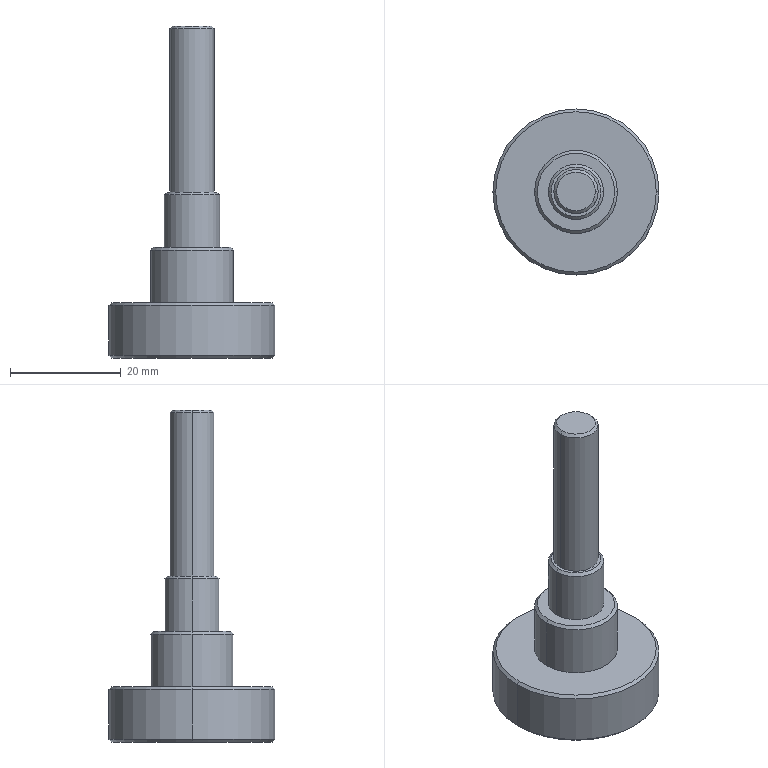Part | SolidWorks | features ICE 3, Chamfer 1, Extrusion 1 | 1 solid | 23 faces | box 30 x 30 x 60 mm | volume 11093 mm3 | cone 10 | cylinder 8 | plane 5 | commonest cylinder face diameters 8 x2 10 x2 15 x2 30 x2
STEP:
#1=CARTESIAN_POINT('',(3.5,0.,60.));
#2=VERTEX_POINT('',#1);
#3=CARTESIAN_POINT('',(-3.5,0.,60.));
#4=VERTEX_POINT('',#3);
#5=CARTESIAN_POINT('',(0.,0.,60.));
#6=DIRECTION('',(0.,0.,1.));
#7=DIRECTION('',(1.,0.,0.));
#8=AXIS2_PLACEMENT_3D('',#5,#6,#7);
#9=CIRCLE('',#8,3.5);
#10=EDGE_CURVE('',#2,#4,#9,.T.);
#11=ORIENTED_EDGE('',*,*,#10,.F.);
#12=CARTESIAN_POINT('',(4.,0.,59.5));
#13=VERTEX_POINT('',#12);
#14=CARTESIAN_POINT('',(3.5,0.,60.));
#15=DIRECTION('',(0.7071,0.,-0.7071));
#16=VECTOR('',#15,1000.);
#17=LINE('',#14,#16);
#18=EDGE_CURVE('',#2,#13,#17,.T.);
#19=ORIENTED_EDGE('',*,*,#18,.T.);
#20=CARTESIAN_POINT('',(-4.,0.,59.5));
#21=VERTEX_POINT('',#20);
#22=CARTESIAN_POINT('',(0.,0.,59.5));
#23=DIRECTION('',(0.,0.,-1.));
#24=DIRECTION('',(1.,0.,0.));
#25=AXIS2_PLACEMENT_3D('',#22,#23,#24);
#26=CIRCLE('',#25,4.);
#27=EDGE_CURVE('',#21,#13,#26,.T.);
#28=ORIENTED_EDGE('',*,*,#27,.F.);
#29=CARTESIAN_POINT('',(-3.5,0.,60.));
#30=DIRECTION('',(-0.7071,0.,-0.7071));
#31=VECTOR('',#30,1000.);
#32=LINE('',#29,#31);
#33=EDGE_CURVE('',#4,#21,#32,.T.);
#34=ORIENTED_EDGE('',*,*,#33,.F.);
#35=EDGE_LOOP('',(#11,#19,#28,#34));
#36=FACE_OUTER_BOUND('',#35,.T.);
#37=CARTESIAN_POINT('',(0.,0.,60.));
#38=DIRECTION('',(0.,0.,-1.));
#39=DIRECTION('',(-1.,0.,0.));
#40=AXIS2_PLACEMENT_3D('',#37,#38,#39);
#41=CONICAL_SURFACE('',#40,3.5,0.7854);
#42=ADVANCED_FACE('',(#36),#41,.T.);
#43=CARTESIAN_POINT('',(4.5,0.,30.));
#44=VERTEX_POINT('',#43);
#45=CARTESIAN_POINT('',(-4.5,0.,30.));
#46=VERTEX_POINT('',#45);
#47=CARTESIAN_POINT('',(0.,0.,30.));
#48=DIRECTION('',(0.,0.,1.));
#49=DIRECTION('',(1.,0.,0.));
#50=AXIS2_PLACEMENT_3D('',#47,#48,#49);
#51=CIRCLE('',#50,4.5);
#52=EDGE_CURVE('',#44,#46,#51,.T.);
#53=ORIENTED_EDGE('',*,*,#52,.F.);
#54=CARTESIAN_POINT('',(5.,0.,29.5));
#55=VERTEX_POINT('',#54);
#56=CARTESIAN_POINT('',(4.5,0.,30.));
#57=DIRECTION('',(0.7071,0.,-0.7071));
#58=VECTOR('',#57,1000.);
#59=LINE('',#56,#58);
#60=EDGE_CURVE('',#44,#55,#59,.T.);
#61=ORIENTED_EDGE('',*,*,#60,.T.);
#62=CARTESIAN_POINT('',(-5.,0.,29.5));
#63=VERTEX_POINT('',#62);
#64=CARTESIAN_POINT('',(0.,0.,29.5));
#65=DIRECTION('',(0.,0.,-1.));
#66=DIRECTION('',(1.,0.,0.));
#67=AXIS2_PLACEMENT_3D('',#64,#65,#66);
#68=CIRCLE('',#67,5.);
#69=EDGE_CURVE('',#63,#55,#68,.T.);
#70=ORIENTED_EDGE('',*,*,#69,.F.);
#71=CARTESIAN_POINT('',(-4.5,0.,30.));
#72=DIRECTION('',(-0.7071,0.,-0.7071));
#73=VECTOR('',#72,1000.);
#74=LINE('',#71,#73);
#75=EDGE_CURVE('',#46,#63,#74,.T.);
#76=ORIENTED_EDGE('',*,*,#75,.F.);
#77=EDGE_LOOP('',(#53,#61,#70,#76));
#78=FACE_OUTER_BOUND('',#77,.T.);
#79=CARTESIAN_POINT('',(0.,0.,30.));
#80=DIRECTION('',(0.,0.,-1.));
#81=DIRECTION('',(-1.,0.,0.));
#82=AXIS2_PLACEMENT_3D('',#79,#80,#81);
#83=CONICAL_SURFACE('',#82,4.5,0.7854);
#84=ADVANCED_FACE('',(#78),#83,.T.);
#85=CARTESIAN_POINT('',(7.,0.,20.));
#86=VERTEX_POINT('',#85);
#87=CARTESIAN_POINT('',(-7.,0.,20.));
#88=VERTEX_POINT('',#87);
#89=CARTESIAN_POINT('',(0.,0.,20.));
#90=DIRECTION('',(0.,0.,1.));
#91=DIRECTION('',(1.,0.,0.));
#92=AXIS2_PLACEMENT_3D('',#89,#90,#91);
#93=CIRCLE('',#92,7.);
#94=EDGE_CURVE('',#86,#88,#93,.T.);
#95=ORIENTED_EDGE('',*,*,#94,.F.);
#96=CARTESIAN_POINT('',(7.5,0.,19.5));
#97=VERTEX_POINT('',#96);
#98=CARTESIAN_POINT('',(7.,0.,20.));
#99=DIRECTION('',(0.7071,0.,-0.7071));
#100=VECTOR('',#99,1000.);
#101=LINE('',#98,#100);
#102=EDGE_CURVE('',#86,#97,#101,.T.);
#103=ORIENTED_EDGE('',*,*,#102,.T.);
#104=CARTESIAN_POINT('',(-7.5,0.,19.5));
#105=VERTEX_POINT('',#104);
#106=CARTESIAN_POINT('',(0.,0.,19.5));
#107=DIRECTION('',(0.,0.,-1.));
#108=DIRECTION('',(1.,0.,0.));
#109=AXIS2_PLACEMENT_3D('',#106,#107,#108);
#110=CIRCLE('',#109,7.5);
#111=EDGE_CURVE('',#105,#97,#110,.T.);
#112=ORIENTED_EDGE('',*,*,#111,.F.);
#113=CARTESIAN_POINT('',(-7.,0.,20.));
#114=DIRECTION('',(-0.7071,0.,-0.7071));
#115=VECTOR('',#114,1000.);
#116=LINE('',#113,#115);
#117=EDGE_CURVE('',#88,#105,#116,.T.);
#118=ORIENTED_EDGE('',*,*,#117,.F.);
#119=EDGE_LOOP('',(#95,#103,#112,#118));
#120=FACE_OUTER_BOUND('',#119,.T.);
#121=CARTESIAN_POINT('',(0.,0.,20.));
#122=DIRECTION('',(0.,0.,-1.));
#123=DIRECTION('',(-1.,0.,0.));
#124=AXIS2_PLACEMENT_3D('',#121,#122,#123);
#125=CONICAL_SURFACE('',#124,7.,0.7854);
#126=ADVANCED_FACE('',(#120),#125,.T.);
#127=CARTESIAN_POINT('',(14.5,0.,10.));
#128=VERTEX_POINT('',#127);
#129=CARTESIAN_POINT('',(-14.5,0.,10.));
#130=VERTEX_POINT('',#129);
#131=CARTESIAN_POINT('',(0.,0.,10.));
#132=DIRECTION('',(0.,0.,1.));
#133=DIRECTION('',(1.,0.,0.));
#134=AXIS2_PLACEMENT_3D('',#131,#132,#133);
#135=CIRCLE('',#134,14.5);
#136=EDGE_CURVE('',#128,#130,#135,.T.);
#137=ORIENTED_EDGE('',*,*,#136,.F.);
#138=CARTESIAN_POINT('',(15.,0.,9.5));
#139=VERTEX_POINT('',#138);
#140=CARTESIAN_POINT('',(14.5,0.,10.));
#141=DIRECTION('',(0.7071,0.,-0.7071));
#142=VECTOR('',#141,1000.);
#143=LINE('',#140,#142);
#144=EDGE_CURVE('',#128,#139,#143,.T.);
#145=ORIENTED_EDGE('',*,*,#144,.T.);
#146=CARTESIAN_POINT('',(-15.,0.,9.5));
#147=VERTEX_POINT('',#146);
#148=CARTESIAN_POINT('',(0.,0.,9.5));
#149=DIRECTION('',(0.,0.,-1.));
#150=DIRECTION('',(1.,0.,0.));
#151=AXIS2_PLACEMENT_3D('',#148,#149,#150);
#152=CIRCLE('',#151,15.);
#153=EDGE_CURVE('',#147,#139,#152,.T.);
#154=ORIENTED_EDGE('',*,*,#153,.F.);
#155=CARTESIAN_POINT('',(-14.5,0.,10.));
#156=DIRECTION('',(-0.7071,0.,-0.7071));
#157=VECTOR('',#156,1000.);
#158=LINE('',#155,#157);
#159=EDGE_CURVE('',#130,#147,#158,.T.);
#160=ORIENTED_EDGE('',*,*,#159,.F.);
#161=EDGE_LOOP('',(#137,#145,#154,#160));
#162=FACE_OUTER_BOUND('',#161,.T.);
#163=CARTESIAN_POINT('',(0.,0.,10.));
#164=DIRECTION('',(0.,0.,-1.));
#165=DIRECTION('',(-1.,0.,0.));
#166=AXIS2_PLACEMENT_3D('',#163,#164,#165);
#167=CONICAL_SURFACE('',#166,14.5,0.7854);
#168=ADVANCED_FACE('',(#162),#167,.T.);
#169=CARTESIAN_POINT('',(-14.5,0.,0.));
#170=VERTEX_POINT('',#169);
#171=CARTESIAN_POINT('',(14.5,0.,0.));
#172=VERTEX_POINT('',#171);
#173=CARTESIAN_POINT('',(0.,0.,0.));
#174=DIRECTION('',(0.,0.,-1.));
#175=DIRECTION('',(1.,0.,0.));
#176=AXIS2_PLACEMENT_3D('',#173,#174,#175);
#177=CIRCLE('',#176,14.5);
#178=EDGE_CURVE('',#170,#172,#177,.T.);
#179=ORIENTED_EDGE('',*,*,#178,.F.);
#180=CARTESIAN_POINT('',(-15.,0.,0.5));
#181=VERTEX_POINT('',#180);
#182=CARTESIAN_POINT('',(-15.,0.,0.5));
#183=DIRECTION('',(-0.7071,0.,0.7071));
#184=VECTOR('',#183,1000.);
#185=LINE('',#182,#184);
#186=EDGE_CURVE('',#170,#181,#185,.T.);
#187=ORIENTED_EDGE('',*,*,#186,.T.);
#188=CARTESIAN_POINT('',(15.,0.,0.5));
#189=VERTEX_POINT('',#188);
#190=CARTESIAN_POINT('',(0.,0.,0.5));
#191=DIRECTION('',(0.,0.,1.));
#192=DIRECTION('',(1.,0.,0.));
#193=AXIS2_PLACEMENT_3D('',#190,#191,#192);
#194=CIRCLE('',#193,15.);
#195=EDGE_CURVE('',#189,#181,#194,.T.);
#196=ORIENTED_EDGE('',*,*,#195,.F.);
#197=CARTESIAN_POINT('',(15.,0.,0.5));
#198=DIRECTION('',(0.7071,0.,0.7071));
#199=VECTOR('',#198,1000.);
#200=LINE('',#197,#199);
#201=EDGE_CURVE('',#172,#189,#200,.T.);
#202=ORIENTED_EDGE('',*,*,#201,.F.);
#203=EDGE_LOOP('',(#179,#187,#196,#202));
#204=FACE_OUTER_BOUND('',#203,.T.);
#205=CARTESIAN_POINT('',(0.,0.,0.5));
#206=DIRECTION('',(0.,0.,1.));
#207=DIRECTION('',(1.,0.,0.));
#208=AXIS2_PLACEMENT_3D('',#205,#206,#207);
#209=CONICAL_SURFACE('',#208,15.,0.7854);
#210=ADVANCED_FACE('',(#204),#209,.T.);
#211=ORIENTED_EDGE('',*,*,#27,.T.);
#212=CARTESIAN_POINT('',(4.,0.,30.));
#213=VERTEX_POINT('',#212);
#214=CARTESIAN_POINT('',(4.,0.,60.));
#215=DIRECTION('',(0.,0.,-1.));
#216=VECTOR('',#215,1000.);
#217=LINE('',#214,#216);
#218=EDGE_CURVE('',#13,#213,#217,.T.);
#219=ORIENTED_EDGE('',*,*,#218,.T.);
#220=CARTESIAN_POINT('',(-4.,0.,30.));
#221=VERTEX_POINT('',#220);
#222=CARTESIAN_POINT('',(0.,0.,30.));
#223=DIRECTION('',(0.,0.,1.));
#224=DIRECTION('',(1.,0.,0.));
#225=AXIS2_PLACEMENT_3D('',#222,#223,#224);
#226=CIRCLE('',#225,4.);
#227=EDGE_CURVE('',#213,#221,#226,.T.);
#228=ORIENTED_EDGE('',*,*,#227,.T.);
#229=CARTESIAN_POINT('',(-4.,0.,60.));
#230=DIRECTION('',(0.,0.,-1.));
#231=VECTOR('',#230,1000.);
#232=LINE('',#229,#231);
#233=EDGE_CURVE('',#21,#221,#232,.T.);
#234=ORIENTED_EDGE('',*,*,#233,.F.);
#235=EDGE_LOOP('',(#211,#219,#228,#234));
#236=FACE_OUTER_BOUND('',#235,.T.);
#237=CARTESIAN_POINT('',(0.,0.,60.));
#238=DIRECTION('',(0.,0.,-1.));
#239=DIRECTION('',(-1.,0.,0.));
#240=AXIS2_PLACEMENT_3D('',#237,#238,#239);
#241=CYLINDRICAL_SURFACE('',#240,4.);
#242=ADVANCED_FACE('',(#236),#241,.T.);
#243=ORIENTED_EDGE('',*,*,#69,.T.);
#244=CARTESIAN_POINT('',(5.,0.,20.));
#245=VERTEX_POINT('',#244);
#246=CARTESIAN_POINT('',(5.,0.,30.));
#247=DIRECTION('',(0.,0.,-1.));
#248=VECTOR('',#247,1000.);
#249=LINE('',#246,#248);
#250=EDGE_CURVE('',#55,#245,#249,.T.);
#251=ORIENTED_EDGE('',*,*,#250,.T.);
#252=CARTESIAN_POINT('',(-5.,0.,20.));
#253=VERTEX_POINT('',#252);
#254=CARTESIAN_POINT('',(0.,0.,20.));
#255=DIRECTION('',(0.,0.,1.));
#256=DIRECTION('',(1.,0.,0.));
#257=AXIS2_PLACEMENT_3D('',#254,#255,#256);
#258=CIRCLE('',#257,5.);
#259=EDGE_CURVE('',#245,#253,#258,.T.);
#260=ORIENTED_EDGE('',*,*,#259,.T.);
#261=CARTESIAN_POINT('',(-5.,0.,30.));
#262=DIRECTION('',(0.,0.,-1.));
#263=VECTOR('',#262,1000.);
#264=LINE('',#261,#263);
#265=EDGE_CURVE('',#63,#253,#264,.T.);
#266=ORIENTED_EDGE('',*,*,#265,.F.);
#267=EDGE_LOOP('',(#243,#251,#260,#266));
#268=FACE_OUTER_BOUND('',#267,.T.);
#269=CARTESIAN_POINT('',(0.,0.,30.));
#270=DIRECTION('',(0.,0.,-1.));
#271=DIRECTION('',(-1.,0.,0.));
#272=AXIS2_PLACEMENT_3D('',#269,#270,#271);
#273=CYLINDRICAL_SURFACE('',#272,5.);
#274=ADVANCED_FACE('',(#268),#273,.T.);
#275=ORIENTED_EDGE('',*,*,#111,.T.);
#276=CARTESIAN_POINT('',(7.5,0.,10.));
#277=VERTEX_POINT('',#276);
#278=CARTESIAN_POINT('',(7.5,0.,20.));
#279=DIRECTION('',(0.,0.,-1.));
#280=VECTOR('',#279,1000.);
#281=LINE('',#278,#280);
#282=EDGE_CURVE('',#97,#277,#281,.T.);
#283=ORIENTED_EDGE('',*,*,#282,.T.);
#284=CARTESIAN_POINT('',(-7.5,0.,10.));
#285=VERTEX_POINT('',#284);
#286=CARTESIAN_POINT('',(0.,0.,10.));
#287=DIRECTION('',(0.,0.,1.));
#288=DIRECTION('',(1.,0.,0.));
#289=AXIS2_PLACEMENT_3D('',#286,#287,#288);
#290=CIRCLE('',#289,7.5);
#291=EDGE_CURVE('',#277,#285,#290,.T.);
#292=ORIENTED_EDGE('',*,*,#291,.T.);
#293=CARTESIAN_POINT('',(-7.5,0.,20.));
#294=DIRECTION('',(0.,0.,-1.));
#295=VECTOR('',#294,1000.);
#296=LINE('',#293,#295);
#297=EDGE_CURVE('',#105,#285,#296,.T.);
#298=ORIENTED_EDGE('',*,*,#297,.F.);
#299=EDGE_LOOP('',(#275,#283,#292,#298));
#300=FACE_OUTER_BOUND('',#299,.T.);
#301=CARTESIAN_POINT('',(0.,0.,20.));
#302=DIRECTION('',(0.,0.,-1.));
#303=DIRECTION('',(-1.,0.,0.));
#304=AXIS2_PLACEMENT_3D('',#301,#302,#303);
#305=CYLINDRICAL_SURFACE('',#304,7.5);
#306=ADVANCED_FACE('',(#300),#305,.T.);
#307=ORIENTED_EDGE('',*,*,#153,.T.);
#308=CARTESIAN_POINT('',(15.,0.,10.));
#309=DIRECTION('',(0.,0.,-1.));
#310=VECTOR('',#309,1000.);
#311=LINE('',#308,#310);
#312=EDGE_CURVE('',#139,#189,#311,.T.);
#313=ORIENTED_EDGE('',*,*,#312,.T.);
#314=ORIENTED_EDGE('',*,*,#195,.T.);
#315=CARTESIAN_POINT('',(-15.,0.,10.));
#316=DIRECTION('',(0.,0.,-1.));
#317=VECTOR('',#316,1000.);
#318=LINE('',#315,#317);
#319=EDGE_CURVE('',#147,#181,#318,.T.);
#320=ORIENTED_EDGE('',*,*,#319,.F.);
#321=EDGE_LOOP('',(#307,#313,#314,#320));
#322=FACE_OUTER_BOUND('',#321,.T.);
#323=CARTESIAN_POINT('',(0.,0.,10.));
#324=DIRECTION('',(0.,0.,-1.));
#325=DIRECTION('',(-1.,0.,0.));
#326=AXIS2_PLACEMENT_3D('',#323,#324,#325);
#327=CYLINDRICAL_SURFACE('',#326,15.);
#328=ADVANCED_FACE('',(#322),#327,.T.);
#329=CARTESIAN_POINT('',(0.,0.,20.));
#330=DIRECTION('',(0.,0.,1.));
#331=DIRECTION('',(1.,0.,0.));
#332=AXIS2_PLACEMENT_3D('',#329,#330,#331);
#333=CIRCLE('',#332,7.);
#334=EDGE_CURVE('',#88,#86,#333,.T.);
#335=ORIENTED_EDGE('',*,*,#334,.T.);
#336=ORIENTED_EDGE('',*,*,#94,.T.);
#337=EDGE_LOOP('',(#335,#336));
#338=FACE_OUTER_BOUND('',#337,.T.);
#339=CARTESIAN_POINT('',(0.,0.,20.));
#340=DIRECTION('',(0.,0.,1.));
#341=DIRECTION('',(1.,0.,0.));
#342=AXIS2_PLACEMENT_3D('',#339,#340,#341);
#343=CIRCLE('',#342,5.);
#344=EDGE_CURVE('',#253,#245,#343,.T.);
#345=ORIENTED_EDGE('',*,*,#344,.F.);
#346=ORIENTED_EDGE('',*,*,#259,.F.);
#347=EDGE_LOOP('',(#345,#346));
#348=FACE_BOUND('',#347,.T.);
#349=CARTESIAN_POINT('',(0.,0.,20.));
#350=DIRECTION('',(0.,0.,1.));
#351=DIRECTION('',(1.,0.,0.));
#352=AXIS2_PLACEMENT_3D('',#349,#350,#351);
#353=PLANE('',#352);
#354=ADVANCED_FACE('',(#338,#348),#353,.T.);
#355=CARTESIAN_POINT('',(0.,0.,10.));
#356=DIRECTION('',(0.,0.,1.));
#357=DIRECTION('',(1.,0.,0.));
#358=AXIS2_PLACEMENT_3D('',#355,#356,#357);
#359=CIRCLE('',#358,14.5);
#360=EDGE_CURVE('',#130,#128,#359,.T.);
#361=ORIENTED_EDGE('',*,*,#360,.T.);
#362=ORIENTED_EDGE('',*,*,#136,.T.);
#363=EDGE_LOOP('',(#361,#362));
#364=FACE_OUTER_BOUND('',#363,.T.);
#365=CARTESIAN_POINT('',(0.,0.,10.));
#366=DIRECTION('',(0.,0.,1.));
#367=DIRECTION('',(1.,0.,0.));
#368=AXIS2_PLACEMENT_3D('',#365,#366,#367);
#369=CIRCLE('',#368,7.5);
#370=EDGE_CURVE('',#285,#277,#369,.T.);
#371=ORIENTED_EDGE('',*,*,#370,.F.);
#372=ORIENTED_EDGE('',*,*,#291,.F.);
#373=EDGE_LOOP('',(#371,#372));
#374=FACE_BOUND('',#373,.T.);
#375=CARTESIAN_POINT('',(0.,0.,10.));
#376=DIRECTION('',(0.,0.,1.));
#377=DIRECTION('',(1.,0.,0.));
#378=AXIS2_PLACEMENT_3D('',#375,#376,#377);
#379=PLANE('',#378);
#380=ADVANCED_FACE('',(#364,#374),#379,.T.);
#381=ORIENTED_EDGE('',*,*,#312,.F.);
#382=CARTESIAN_POINT('',(0.,0.,9.5));
#383=DIRECTION('',(0.,0.,-1.));
#384=DIRECTION('',(1.,0.,0.));
#385=AXIS2_PLACEMENT_3D('',#382,#383,#384);
#386=CIRCLE('',#385,15.);
#387=EDGE_CURVE('',#139,#147,#386,.T.);
#388=ORIENTED_EDGE('',*,*,#387,.T.);
#389=ORIENTED_EDGE('',*,*,#319,.T.);
#390=CARTESIAN_POINT('',(0.,0.,0.5));
#391=DIRECTION('',(0.,0.,1.));
#392=DIRECTION('',(1.,0.,0.));
#393=AXIS2_PLACEMENT_3D('',#390,#391,#392);
#394=CIRCLE('',#393,15.);
#395=EDGE_CURVE('',#181,#189,#394,.T.);
#396=ORIENTED_EDGE('',*,*,#395,.T.);
#397=EDGE_LOOP('',(#381,#388,#389,#396));
#398=FACE_OUTER_BOUND('',#397,.T.);
#399=CARTESIAN_POINT('',(0.,0.,10.));
#400=DIRECTION('',(0.,0.,-1.));
#401=DIRECTION('',(-1.,0.,0.));
#402=AXIS2_PLACEMENT_3D('',#399,#400,#401);
#403=CYLINDRICAL_SURFACE('',#402,15.);
#404=ADVANCED_FACE('',(#398),#403,.T.);
#405=CARTESIAN_POINT('',(0.,0.,0.));
#406=DIRECTION('',(0.,0.,-1.));
#407=DIRECTION('',(1.,0.,0.));
#408=AXIS2_PLACEMENT_3D('',#405,#406,#407);
#409=CIRCLE('',#408,14.5);
#410=EDGE_CURVE('',#172,#170,#409,.T.);
#411=ORIENTED_EDGE('',*,*,#410,.T.);
#412=ORIENTED_EDGE('',*,*,#178,.T.);
#413=EDGE_LOOP('',(#411,#412));
#414=FACE_OUTER_BOUND('',#413,.T.);
#415=CARTESIAN_POINT('',(0.,0.,0.));
#416=DIRECTION('',(0.,0.,1.));
#417=DIRECTION('',(1.,0.,0.));
#418=AXIS2_PLACEMENT_3D('',#415,#416,#417);
#419=PLANE('',#418);
#420=ADVANCED_FACE('',(#414),#419,.F.);
#421=ORIENTED_EDGE('',*,*,#282,.F.);
#422=CARTESIAN_POINT('',(0.,0.,19.5));
#423=DIRECTION('',(0.,0.,-1.));
#424=DIRECTION('',(1.,0.,0.));
#425=AXIS2_PLACEMENT_3D('',#422,#423,#424);
#426=CIRCLE('',#425,7.5);
#427=EDGE_CURVE('',#97,#105,#426,.T.);
#428=ORIENTED_EDGE('',*,*,#427,.T.);
#429=ORIENTED_EDGE('',*,*,#297,.T.);
#430=ORIENTED_EDGE('',*,*,#370,.T.);
#431=EDGE_LOOP('',(#421,#428,#429,#430));
#432=FACE_OUTER_BOUND('',#431,.T.);
#433=CARTESIAN_POINT('',(0.,0.,20.));
#434=DIRECTION('',(0.,0.,-1.));
#435=DIRECTION('',(-1.,0.,0.));
#436=AXIS2_PLACEMENT_3D('',#433,#434,#435);
#437=CYLINDRICAL_SURFACE('',#436,7.5);
#438=ADVANCED_FACE('',(#432),#437,.T.);
#439=CARTESIAN_POINT('',(0.,0.,30.));
#440=DIRECTION('',(0.,0.,1.));
#441=DIRECTION('',(1.,0.,0.));
#442=AXIS2_PLACEMENT_3D('',#439,#440,#441);
#443=CIRCLE('',#442,4.5);
#444=EDGE_CURVE('',#46,#44,#443,.T.);
#445=ORIENTED_EDGE('',*,*,#444,.T.);
#446=ORIENTED_EDGE('',*,*,#52,.T.);
#447=EDGE_LOOP('',(#445,#446));
#448=FACE_OUTER_BOUND('',#447,.T.);
#449=CARTESIAN_POINT('',(0.,0.,30.));
#450=DIRECTION('',(0.,0.,1.));
#451=DIRECTION('',(1.,0.,0.));
#452=AXIS2_PLACEMENT_3D('',#449,#450,#451);
#453=CIRCLE('',#452,4.);
#454=EDGE_CURVE('',#221,#213,#453,.T.);
#455=ORIENTED_EDGE('',*,*,#454,.F.);
#456=ORIENTED_EDGE('',*,*,#227,.F.);
#457=EDGE_LOOP('',(#455,#456));
#458=FACE_BOUND('',#457,.T.);
#459=CARTESIAN_POINT('',(0.,0.,30.));
#460=DIRECTION('',(0.,0.,1.));
#461=DIRECTION('',(1.,0.,0.));
#462=AXIS2_PLACEMENT_3D('',#459,#460,#461);
#463=PLANE('',#462);
#464=ADVANCED_FACE('',(#448,#458),#463,.T.);
#465=ORIENTED_EDGE('',*,*,#250,.F.);
#466=CARTESIAN_POINT('',(0.,0.,29.5));
#467=DIRECTION('',(0.,0.,-1.));
#468=DIRECTION('',(1.,0.,0.));
#469=AXIS2_PLACEMENT_3D('',#466,#467,#468);
#470=CIRCLE('',#469,5.);
#471=EDGE_CURVE('',#55,#63,#470,.T.);
#472=ORIENTED_EDGE('',*,*,#471,.T.);
#473=ORIENTED_EDGE('',*,*,#265,.T.);
#474=ORIENTED_EDGE('',*,*,#344,.T.);
#475=EDGE_LOOP('',(#465,#472,#473,#474));
#476=FACE_OUTER_BOUND('',#475,.T.);
#477=CARTESIAN_POINT('',(0.,0.,30.));
#478=DIRECTION('',(0.,0.,-1.));
#479=DIRECTION('',(-1.,0.,0.));
#480=AXIS2_PLACEMENT_3D('',#477,#478,#479);
#481=CYLINDRICAL_SURFACE('',#480,5.);
#482=ADVANCED_FACE('',(#476),#481,.T.);
#483=CARTESIAN_POINT('',(0.,0.,60.));
#484=DIRECTION('',(0.,0.,1.));
#485=DIRECTION('',(1.,0.,0.));
#486=AXIS2_PLACEMENT_3D('',#483,#484,#485);
#487=CIRCLE('',#486,3.5);
#488=EDGE_CURVE('',#4,#2,#487,.T.);
#489=ORIENTED_EDGE('',*,*,#488,.T.);
#490=ORIENTED_EDGE('',*,*,#10,.T.);
#491=EDGE_LOOP('',(#489,#490));
#492=FACE_OUTER_BOUND('',#491,.T.);
#493=CARTESIAN_POINT('',(0.,0.,60.));
#494=DIRECTION('',(0.,0.,1.));
#495=DIRECTION('',(1.,0.,0.));
#496=AXIS2_PLACEMENT_3D('',#493,#494,#495);
#497=PLANE('',#496);
#498=ADVANCED_FACE('',(#492),#497,.T.);
#499=ORIENTED_EDGE('',*,*,#218,.F.);
#500=CARTESIAN_POINT('',(0.,0.,59.5));
#501=DIRECTION('',(0.,0.,-1.));
#502=DIRECTION('',(1.,0.,0.));
#503=AXIS2_PLACEMENT_3D('',#500,#501,#502);
#504=CIRCLE('',#503,4.);
#505=EDGE_CURVE('',#13,#21,#504,.T.);
#506=ORIENTED_EDGE('',*,*,#505,.T.);
#507=ORIENTED_EDGE('',*,*,#233,.T.);
#508=ORIENTED_EDGE('',*,*,#454,.T.);
#509=EDGE_LOOP('',(#499,#506,#507,#508));
#510=FACE_OUTER_BOUND('',#509,.T.);
#511=CARTESIAN_POINT('',(0.,0.,60.));
#512=DIRECTION('',(0.,0.,-1.));
#513=DIRECTION('',(-1.,0.,0.));
#514=AXIS2_PLACEMENT_3D('',#511,#512,#513);
#515=CYLINDRICAL_SURFACE('',#514,4.);
#516=ADVANCED_FACE('',(#510),#515,.T.);
#517=ORIENTED_EDGE('',*,*,#186,.F.);
#518=ORIENTED_EDGE('',*,*,#410,.F.);
#519=ORIENTED_EDGE('',*,*,#201,.T.);
#520=ORIENTED_EDGE('',*,*,#395,.F.);
#521=EDGE_LOOP('',(#517,#518,#519,#520));
#522=FACE_OUTER_BOUND('',#521,.T.);
#523=CARTESIAN_POINT('',(0.,0.,0.5));
#524=DIRECTION('',(0.,0.,1.));
#525=DIRECTION('',(1.,0.,0.));
#526=AXIS2_PLACEMENT_3D('',#523,#524,#525);
#527=CONICAL_SURFACE('',#526,15.,0.7854);
#528=ADVANCED_FACE('',(#522),#527,.T.);
#529=ORIENTED_EDGE('',*,*,#144,.F.);
#530=ORIENTED_EDGE('',*,*,#360,.F.);
#531=ORIENTED_EDGE('',*,*,#159,.T.);
#532=ORIENTED_EDGE('',*,*,#387,.F.);
#533=EDGE_LOOP('',(#529,#530,#531,#532));
#534=FACE_OUTER_BOUND('',#533,.T.);
#535=CARTESIAN_POINT('',(0.,0.,10.));
#536=DIRECTION('',(0.,0.,-1.));
#537=DIRECTION('',(-1.,0.,0.));
#538=AXIS2_PLACEMENT_3D('',#535,#536,#537);
#539=CONICAL_SURFACE('',#538,14.5,0.7854);
#540=ADVANCED_FACE('',(#534),#539,.T.);
#541=ORIENTED_EDGE('',*,*,#102,.F.);
#542=ORIENTED_EDGE('',*,*,#334,.F.);
#543=ORIENTED_EDGE('',*,*,#117,.T.);
#544=ORIENTED_EDGE('',*,*,#427,.F.);
#545=EDGE_LOOP('',(#541,#542,#543,#544));
#546=FACE_OUTER_BOUND('',#545,.T.);
#547=CARTESIAN_POINT('',(0.,0.,20.));
#548=DIRECTION('',(0.,0.,-1.));
#549=DIRECTION('',(-1.,0.,0.));
#550=AXIS2_PLACEMENT_3D('',#547,#548,#549);
#551=CONICAL_SURFACE('',#550,7.,0.7854);
#552=ADVANCED_FACE('',(#546),#551,.T.);
#553=ORIENTED_EDGE('',*,*,#60,.F.);
#554=ORIENTED_EDGE('',*,*,#444,.F.);
#555=ORIENTED_EDGE('',*,*,#75,.T.);
#556=ORIENTED_EDGE('',*,*,#471,.F.);
#557=EDGE_LOOP('',(#553,#554,#555,#556));
#558=FACE_OUTER_BOUND('',#557,.T.);
#559=CARTESIAN_POINT('',(0.,0.,30.));
#560=DIRECTION('',(0.,0.,-1.));
#561=DIRECTION('',(-1.,0.,0.));
#562=AXIS2_PLACEMENT_3D('',#559,#560,#561);
#563=CONICAL_SURFACE('',#562,4.5,0.7854);
#564=ADVANCED_FACE('',(#558),#563,.T.);
#565=ORIENTED_EDGE('',*,*,#18,.F.);
#566=ORIENTED_EDGE('',*,*,#488,.F.);
#567=ORIENTED_EDGE('',*,*,#33,.T.);
#568=ORIENTED_EDGE('',*,*,#505,.F.);
#569=EDGE_LOOP('',(#565,#566,#567,#568));
#570=FACE_OUTER_BOUND('',#569,.T.);
#571=CARTESIAN_POINT('',(0.,0.,60.));
#572=DIRECTION('',(0.,0.,-1.));
#573=DIRECTION('',(-1.,0.,0.));
#574=AXIS2_PLACEMENT_3D('',#571,#572,#573);
#575=CONICAL_SURFACE('',#574,3.5,0.7854);
#576=ADVANCED_FACE('',(#570),#575,.T.);
#577=CLOSED_SHELL('',(#42,#84,#126,#168,#210,#242,#274,#306,#328,#354,#380,#404,#420,#438,#464,#482,#498,#516,#528,#540,#552,#564,#576));
#578=MANIFOLD_SOLID_BREP('',#577);
#579=CARTESIAN_POINT('',(0.,0.,0.));
#580=DIRECTION('',(0.,0.,1.));
#581=DIRECTION('',(1.,0.,0.));
#582=AXIS2_PLACEMENT_3D('',#579,#580,#581);
#583=(LENGTH_UNIT()NAMED_UNIT(*)SI_UNIT(.MILLI.,.METRE.));
#584=UNCERTAINTY_MEASURE_WITH_UNIT(LENGTH_MEASURE(0.00001),#583,'','');
#585=(NAMED_UNIT(*)PLANE_ANGLE_UNIT()SI_UNIT($,.RADIAN.));
#586=(NAMED_UNIT(*)SI_UNIT($,.STERADIAN.)SOLID_ANGLE_UNIT());
#587=(GEOMETRIC_REPRESENTATION_CONTEXT(3)GLOBAL_UNCERTAINTY_ASSIGNED_CONTEXT((#584))GLOBAL_UNIT_ASSIGNED_CONTEXT((#583,#585,#586))REPRESENTATION_CONTEXT('',''));
#588=ADVANCED_BREP_SHAPE_REPRESENTATION('',(#578,#582),#587);